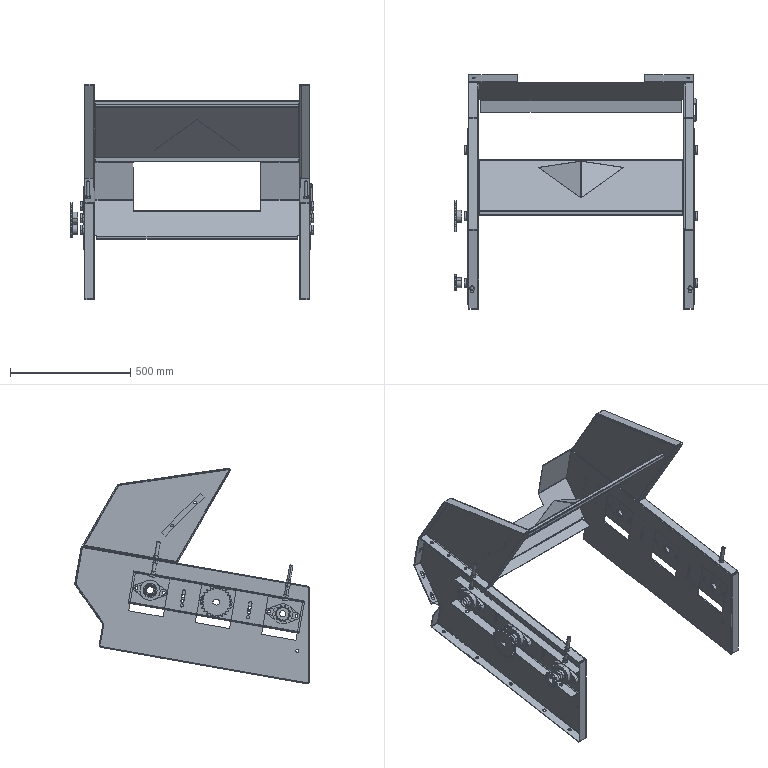Part | SolidWorks | features LayoutProfileFeature 1 | 46 solids | 1905 faces | box 1011 x 975.086 x 897.064 mm | volume 6794534 mm3 | cylinder 719 | plane 696 | spline 262 | cone 228 | commonest cylinder face diameters 13 x115 26.518 x76 16.697 x50 38 x48 10.262 x46 15 x40